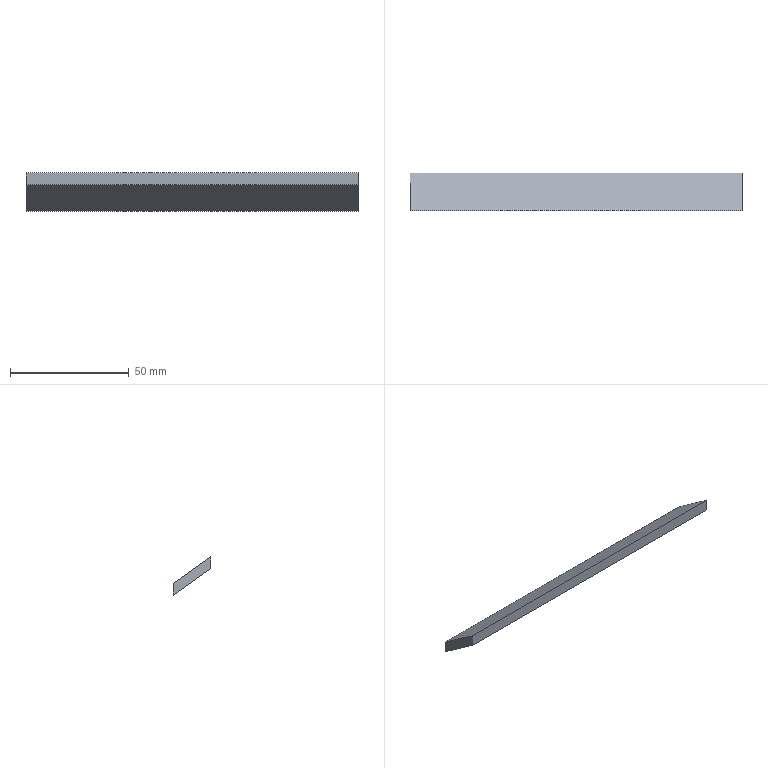Part | STEP file | 06-35 Front-rear dovetail press strip | 1 solid | 6 faces | box 140 x 16 x 16.203 mm | volume 11200 mm3 | plane 6
STEP:
#1=CARTESIAN_POINT('',(0.,0.,0.));
#2=DIRECTION('',(0.,0.,1.));
#3=DIRECTION('',(1.,0.,0.));
#4=AXIS2_PLACEMENT_3D('',#1,#2,#3);
#5=CARTESIAN_POINT('',(140.,0.,-0.000000002));
#6=VERTEX_POINT('',#5);
#7=CARTESIAN_POINT('',(0.,0.,-0.000000001));
#8=VERTEX_POINT('',#7);
#9=CARTESIAN_POINT('',(70.,0.,0.));
#10=DIRECTION('',(-1.,0.,0.));
#11=VECTOR('',#10,1.);
#12=LINE('',#9,#11);
#13=CARTESIAN_POINT('',(0.,0.,0.));
#14=DIRECTION('',(0.,-0.5736,-0.8192));
#15=DIRECTION('',(0.,0.8192,-0.5736));
#16=AXIS2_PLACEMENT_3D('',#13,#14,#15);
#17=PLANE('',#16);
#18=CARTESIAN_POINT('',(0.,70.));
#19=DIRECTION('',(0.,-1.));
#20=VECTOR('',#19,1.);
#21=LINE('',#18,#20);
#22=(GEOMETRIC_REPRESENTATION_CONTEXT(2)PARAMETRIC_REPRESENTATION_CONTEXT()REPRESENTATION_CONTEXT('',''));
#23=DEFINITIONAL_REPRESENTATION('',(#21),#22);
#24=PCURVE('',#17,#23);
#25=CARTESIAN_POINT('',(0.,0.,-5.));
#26=DIRECTION('',(0.,1.,0.));
#27=DIRECTION('',(0.,0.,1.));
#28=AXIS2_PLACEMENT_3D('',#25,#26,#27);
#29=PLANE('',#28);
#30=CARTESIAN_POINT('',(5.,70.));
#31=DIRECTION('',(0.,-1.));
#32=VECTOR('',#31,1.);
#33=LINE('',#30,#32);
#34=(GEOMETRIC_REPRESENTATION_CONTEXT(2)PARAMETRIC_REPRESENTATION_CONTEXT()REPRESENTATION_CONTEXT('',''));
#35=DEFINITIONAL_REPRESENTATION('',(#33),#34);
#36=PCURVE('',#29,#35);
#37=SURFACE_CURVE('',#12,(#24,#36),.PCURVE_S1.);
#38=EDGE_CURVE('',#6,#8,#37,.T.);
#39=ORIENTED_EDGE('',*,*,#38,.F.);
#40=CARTESIAN_POINT('',(140.,16.,-11.203));
#41=VERTEX_POINT('',#40);
#42=CARTESIAN_POINT('',(140.,8.,-5.602));
#43=DIRECTION('',(0.,-0.8192,0.5736));
#44=VECTOR('',#43,1.);
#45=LINE('',#42,#44);
#46=CARTESIAN_POINT('',(9.766,140.));
#47=DIRECTION('',(-1.,0.));
#48=VECTOR('',#47,1.);
#49=LINE('',#46,#48);
#50=(GEOMETRIC_REPRESENTATION_CONTEXT(2)PARAMETRIC_REPRESENTATION_CONTEXT()REPRESENTATION_CONTEXT('',''));
#51=DEFINITIONAL_REPRESENTATION('',(#49),#50);
#52=PCURVE('',#17,#51);
#53=CARTESIAN_POINT('',(140.,0.,0.09722));
#54=DIRECTION('',(1.,0.,0.));
#55=DIRECTION('',(0.,0.,-1.));
#56=AXIS2_PLACEMENT_3D('',#53,#54,#55);
#57=PLANE('',#56);
#58=CARTESIAN_POINT('',(5.699,8.));
#59=DIRECTION('',(-0.5736,-0.8192));
#60=VECTOR('',#59,1.);
#61=LINE('',#58,#60);
#62=(GEOMETRIC_REPRESENTATION_CONTEXT(2)PARAMETRIC_REPRESENTATION_CONTEXT()REPRESENTATION_CONTEXT('',''));
#63=DEFINITIONAL_REPRESENTATION('',(#61),#62);
#64=PCURVE('',#57,#63);
#65=SURFACE_CURVE('',#45,(#52,#64),.PCURVE_S1.);
#66=EDGE_CURVE('',#41,#6,#65,.T.);
#67=ORIENTED_EDGE('',*,*,#66,.F.);
#68=CARTESIAN_POINT('',(0.,16.,-11.203));
#69=VERTEX_POINT('',#68);
#70=CARTESIAN_POINT('',(70.,16.,-11.203));
#71=DIRECTION('',(1.,0.,0.));
#72=VECTOR('',#71,1.);
#73=LINE('',#70,#72);
#74=CARTESIAN_POINT('',(19.532,70.));
#75=DIRECTION('',(0.,1.));
#76=VECTOR('',#75,1.);
#77=LINE('',#74,#76);
#78=(GEOMETRIC_REPRESENTATION_CONTEXT(2)PARAMETRIC_REPRESENTATION_CONTEXT()REPRESENTATION_CONTEXT('',''));
#79=DEFINITIONAL_REPRESENTATION('',(#77),#78);
#80=PCURVE('',#17,#79);
#81=CARTESIAN_POINT('',(0.,16.,-11.203));
#82=DIRECTION('',(0.,-1.,0.));
#83=DIRECTION('',(0.,0.,-1.));
#84=AXIS2_PLACEMENT_3D('',#81,#82,#83);
#85=PLANE('',#84);
#86=CARTESIAN_POINT('',(0.,70.));
#87=DIRECTION('',(0.,1.));
#88=VECTOR('',#87,1.);
#89=LINE('',#86,#88);
#90=(GEOMETRIC_REPRESENTATION_CONTEXT(2)PARAMETRIC_REPRESENTATION_CONTEXT()REPRESENTATION_CONTEXT('',''));
#91=DEFINITIONAL_REPRESENTATION('',(#89),#90);
#92=PCURVE('',#85,#91);
#93=SURFACE_CURVE('',#73,(#80,#92),.PCURVE_S1.);
#94=EDGE_CURVE('',#69,#41,#93,.T.);
#95=ORIENTED_EDGE('',*,*,#94,.F.);
#96=CARTESIAN_POINT('',(0.,8.,-5.602));
#97=DIRECTION('',(0.,0.8192,-0.5736));
#98=VECTOR('',#97,1.);
#99=LINE('',#96,#98);
#100=CARTESIAN_POINT('',(9.766,0.));
#101=DIRECTION('',(1.,0.));
#102=VECTOR('',#101,1.);
#103=LINE('',#100,#102);
#104=(GEOMETRIC_REPRESENTATION_CONTEXT(2)PARAMETRIC_REPRESENTATION_CONTEXT()REPRESENTATION_CONTEXT('',''));
#105=DEFINITIONAL_REPRESENTATION('',(#103),#104);
#106=PCURVE('',#17,#105);
#107=CARTESIAN_POINT('',(0.,0.,0.09722));
#108=DIRECTION('',(1.,0.,0.));
#109=DIRECTION('',(0.,0.,-1.));
#110=AXIS2_PLACEMENT_3D('',#107,#108,#109);
#111=PLANE('',#110);
#112=CARTESIAN_POINT('',(5.699,8.));
#113=DIRECTION('',(0.5736,0.8192));
#114=VECTOR('',#113,1.);
#115=LINE('',#112,#114);
#116=(GEOMETRIC_REPRESENTATION_CONTEXT(2)PARAMETRIC_REPRESENTATION_CONTEXT()REPRESENTATION_CONTEXT('',''));
#117=DEFINITIONAL_REPRESENTATION('',(#115),#116);
#118=PCURVE('',#111,#117);
#119=SURFACE_CURVE('',#99,(#106,#118),.PCURVE_S1.);
#120=EDGE_CURVE('',#8,#69,#119,.T.);
#121=ORIENTED_EDGE('',*,*,#120,.F.);
#122=EDGE_LOOP('',(#39,#67,#95,#121));
#123=FACE_BOUND('',#122,.T.);
#124=ADVANCED_FACE('',(#123),#17,.F.);
#125=CARTESIAN_POINT('',(0.,16.,-16.203));
#126=VERTEX_POINT('',#125);
#127=CARTESIAN_POINT('',(0.,16.,-8.102));
#128=DIRECTION('',(0.,0.,1.));
#129=VECTOR('',#128,1.);
#130=LINE('',#127,#129);
#131=CARTESIAN_POINT('',(8.199,16.));
#132=DIRECTION('',(-1.,0.));
#133=VECTOR('',#132,1.);
#134=LINE('',#131,#133);
#135=(GEOMETRIC_REPRESENTATION_CONTEXT(2)PARAMETRIC_REPRESENTATION_CONTEXT()REPRESENTATION_CONTEXT('',''));
#136=DEFINITIONAL_REPRESENTATION('',(#134),#135);
#137=PCURVE('',#111,#136);
#138=CARTESIAN_POINT('',(-3.102,0.));
#139=DIRECTION('',(-1.,0.));
#140=VECTOR('',#139,1.);
#141=LINE('',#138,#140);
#142=(GEOMETRIC_REPRESENTATION_CONTEXT(2)PARAMETRIC_REPRESENTATION_CONTEXT()REPRESENTATION_CONTEXT('',''));
#143=DEFINITIONAL_REPRESENTATION('',(#141),#142);
#144=PCURVE('',#85,#143);
#145=SURFACE_CURVE('',#130,(#137,#144),.PCURVE_S1.);
#146=EDGE_CURVE('',#126,#69,#145,.T.);
#147=ORIENTED_EDGE('',*,*,#146,.F.);
#148=CARTESIAN_POINT('',(0.,0.,-5.));
#149=VERTEX_POINT('',#148);
#150=CARTESIAN_POINT('',(0.,16.,-16.203));
#151=DIRECTION('',(0.,0.8192,-0.5736));
#152=VECTOR('',#151,1.);
#153=LINE('',#150,#152);
#154=CARTESIAN_POINT('',(16.301,16.));
#155=DIRECTION('',(0.5736,0.8192));
#156=VECTOR('',#155,1.);
#157=LINE('',#154,#156);
#158=(GEOMETRIC_REPRESENTATION_CONTEXT(2)PARAMETRIC_REPRESENTATION_CONTEXT()REPRESENTATION_CONTEXT('',''));
#159=DEFINITIONAL_REPRESENTATION('',(#157),#158);
#160=PCURVE('',#111,#159);
#161=CARTESIAN_POINT('',(0.,16.,-16.203));
#162=DIRECTION('',(0.,0.5736,0.8192));
#163=DIRECTION('',(0.,-0.8192,0.5736));
#164=AXIS2_PLACEMENT_3D('',#161,#162,#163);
#165=PLANE('',#164);
#166=CARTESIAN_POINT('',(0.,0.));
#167=DIRECTION('',(-1.,0.));
#168=VECTOR('',#167,1.);
#169=LINE('',#166,#168);
#170=(GEOMETRIC_REPRESENTATION_CONTEXT(2)PARAMETRIC_REPRESENTATION_CONTEXT()REPRESENTATION_CONTEXT('',''));
#171=DEFINITIONAL_REPRESENTATION('',(#169),#170);
#172=PCURVE('',#165,#171);
#173=SURFACE_CURVE('',#153,(#160,#172),.PCURVE_S1.);
#174=EDGE_CURVE('',#149,#126,#173,.T.);
#175=ORIENTED_EDGE('',*,*,#174,.F.);
#176=CARTESIAN_POINT('',(0.,0.,-8.102));
#177=DIRECTION('',(0.,0.,-1.));
#178=VECTOR('',#177,1.);
#179=LINE('',#176,#178);
#180=CARTESIAN_POINT('',(8.199,0.));
#181=DIRECTION('',(1.,0.));
#182=VECTOR('',#181,1.);
#183=LINE('',#180,#182);
#184=(GEOMETRIC_REPRESENTATION_CONTEXT(2)PARAMETRIC_REPRESENTATION_CONTEXT()REPRESENTATION_CONTEXT('',''));
#185=DEFINITIONAL_REPRESENTATION('',(#183),#184);
#186=PCURVE('',#111,#185);
#187=CARTESIAN_POINT('',(-3.102,0.));
#188=DIRECTION('',(-1.,0.));
#189=VECTOR('',#188,1.);
#190=LINE('',#187,#189);
#191=(GEOMETRIC_REPRESENTATION_CONTEXT(2)PARAMETRIC_REPRESENTATION_CONTEXT()REPRESENTATION_CONTEXT('',''));
#192=DEFINITIONAL_REPRESENTATION('',(#190),#191);
#193=PCURVE('',#29,#192);
#194=SURFACE_CURVE('',#179,(#186,#193),.PCURVE_S1.);
#195=EDGE_CURVE('',#8,#149,#194,.T.);
#196=ORIENTED_EDGE('',*,*,#195,.F.);
#197=ORIENTED_EDGE('',*,*,#120,.T.);
#198=EDGE_LOOP('',(#147,#175,#196,#197));
#199=FACE_BOUND('',#198,.T.);
#200=ADVANCED_FACE('',(#199),#111,.F.);
#201=CARTESIAN_POINT('',(140.,0.,-5.));
#202=VERTEX_POINT('',#201);
#203=CARTESIAN_POINT('',(70.,0.,-5.));
#204=DIRECTION('',(-1.,0.,0.));
#205=VECTOR('',#204,1.);
#206=LINE('',#203,#205);
#207=CARTESIAN_POINT('',(0.,70.));
#208=DIRECTION('',(0.,-1.));
#209=VECTOR('',#208,1.);
#210=LINE('',#207,#209);
#211=(GEOMETRIC_REPRESENTATION_CONTEXT(2)PARAMETRIC_REPRESENTATION_CONTEXT()REPRESENTATION_CONTEXT('',''));
#212=DEFINITIONAL_REPRESENTATION('',(#210),#211);
#213=PCURVE('',#29,#212);
#214=CARTESIAN_POINT('',(19.532,70.));
#215=DIRECTION('',(0.,-1.));
#216=VECTOR('',#215,1.);
#217=LINE('',#214,#216);
#218=(GEOMETRIC_REPRESENTATION_CONTEXT(2)PARAMETRIC_REPRESENTATION_CONTEXT()REPRESENTATION_CONTEXT('',''));
#219=DEFINITIONAL_REPRESENTATION('',(#217),#218);
#220=PCURVE('',#165,#219);
#221=SURFACE_CURVE('',#206,(#213,#220),.PCURVE_S1.);
#222=EDGE_CURVE('',#202,#149,#221,.T.);
#223=ORIENTED_EDGE('',*,*,#222,.F.);
#224=CARTESIAN_POINT('',(140.,0.,-2.5));
#225=DIRECTION('',(0.,0.,-1.));
#226=VECTOR('',#225,1.);
#227=LINE('',#224,#226);
#228=CARTESIAN_POINT('',(2.5,140.));
#229=DIRECTION('',(-1.,0.));
#230=VECTOR('',#229,1.);
#231=LINE('',#228,#230);
#232=(GEOMETRIC_REPRESENTATION_CONTEXT(2)PARAMETRIC_REPRESENTATION_CONTEXT()REPRESENTATION_CONTEXT('',''));
#233=DEFINITIONAL_REPRESENTATION('',(#231),#232);
#234=PCURVE('',#29,#233);
#235=CARTESIAN_POINT('',(2.597,0.));
#236=DIRECTION('',(1.,0.));
#237=VECTOR('',#236,1.);
#238=LINE('',#235,#237);
#239=(GEOMETRIC_REPRESENTATION_CONTEXT(2)PARAMETRIC_REPRESENTATION_CONTEXT()REPRESENTATION_CONTEXT('',''));
#240=DEFINITIONAL_REPRESENTATION('',(#238),#239);
#241=PCURVE('',#57,#240);
#242=SURFACE_CURVE('',#227,(#234,#241),.PCURVE_S1.);
#243=EDGE_CURVE('',#6,#202,#242,.T.);
#244=ORIENTED_EDGE('',*,*,#243,.F.);
#245=ORIENTED_EDGE('',*,*,#38,.T.);
#246=ORIENTED_EDGE('',*,*,#195,.T.);
#247=EDGE_LOOP('',(#223,#244,#245,#246));
#248=FACE_BOUND('',#247,.T.);
#249=ADVANCED_FACE('',(#248),#29,.F.);
#250=CARTESIAN_POINT('',(140.,16.,-16.203));
#251=VERTEX_POINT('',#250);
#252=CARTESIAN_POINT('',(140.,0.,-5.));
#253=DIRECTION('',(0.,0.8192,-0.5736));
#254=VECTOR('',#253,1.);
#255=LINE('',#252,#254);
#256=CARTESIAN_POINT('',(5.097,0.));
#257=DIRECTION('',(0.5736,0.8192));
#258=VECTOR('',#257,1.);
#259=LINE('',#256,#258);
#260=(GEOMETRIC_REPRESENTATION_CONTEXT(2)PARAMETRIC_REPRESENTATION_CONTEXT()REPRESENTATION_CONTEXT('',''));
#261=DEFINITIONAL_REPRESENTATION('',(#259),#260);
#262=PCURVE('',#57,#261);
#263=CARTESIAN_POINT('',(19.532,140.));
#264=DIRECTION('',(-1.,0.));
#265=VECTOR('',#264,1.);
#266=LINE('',#263,#265);
#267=(GEOMETRIC_REPRESENTATION_CONTEXT(2)PARAMETRIC_REPRESENTATION_CONTEXT()REPRESENTATION_CONTEXT('',''));
#268=DEFINITIONAL_REPRESENTATION('',(#266),#267);
#269=PCURVE('',#165,#268);
#270=SURFACE_CURVE('',#255,(#262,#269),.PCURVE_S1.);
#271=EDGE_CURVE('',#202,#251,#270,.T.);
#272=ORIENTED_EDGE('',*,*,#271,.T.);
#273=CARTESIAN_POINT('',(140.,16.,-8.102));
#274=DIRECTION('',(0.,0.,1.));
#275=VECTOR('',#274,1.);
#276=LINE('',#273,#275);
#277=CARTESIAN_POINT('',(8.199,16.));
#278=DIRECTION('',(-1.,0.));
#279=VECTOR('',#278,1.);
#280=LINE('',#277,#279);
#281=(GEOMETRIC_REPRESENTATION_CONTEXT(2)PARAMETRIC_REPRESENTATION_CONTEXT()REPRESENTATION_CONTEXT('',''));
#282=DEFINITIONAL_REPRESENTATION('',(#280),#281);
#283=PCURVE('',#57,#282);
#284=CARTESIAN_POINT('',(-3.102,140.));
#285=DIRECTION('',(-1.,0.));
#286=VECTOR('',#285,1.);
#287=LINE('',#284,#286);
#288=(GEOMETRIC_REPRESENTATION_CONTEXT(2)PARAMETRIC_REPRESENTATION_CONTEXT()REPRESENTATION_CONTEXT('',''));
#289=DEFINITIONAL_REPRESENTATION('',(#287),#288);
#290=PCURVE('',#85,#289);
#291=SURFACE_CURVE('',#276,(#283,#290),.PCURVE_S1.);
#292=EDGE_CURVE('',#251,#41,#291,.T.);
#293=ORIENTED_EDGE('',*,*,#292,.T.);
#294=ORIENTED_EDGE('',*,*,#66,.T.);
#295=ORIENTED_EDGE('',*,*,#243,.T.);
#296=EDGE_LOOP('',(#272,#293,#294,#295));
#297=FACE_BOUND('',#296,.T.);
#298=ADVANCED_FACE('',(#297),#57,.T.);
#299=ORIENTED_EDGE('',*,*,#94,.T.);
#300=ORIENTED_EDGE('',*,*,#292,.F.);
#301=CARTESIAN_POINT('',(70.,16.,-16.203));
#302=DIRECTION('',(1.,0.,0.));
#303=VECTOR('',#302,1.);
#304=LINE('',#301,#303);
#305=CARTESIAN_POINT('',(5.,70.));
#306=DIRECTION('',(0.,1.));
#307=VECTOR('',#306,1.);
#308=LINE('',#305,#307);
#309=(GEOMETRIC_REPRESENTATION_CONTEXT(2)PARAMETRIC_REPRESENTATION_CONTEXT()REPRESENTATION_CONTEXT('',''));
#310=DEFINITIONAL_REPRESENTATION('',(#308),#309);
#311=PCURVE('',#85,#310);
#312=CARTESIAN_POINT('',(0.,70.));
#313=DIRECTION('',(0.,1.));
#314=VECTOR('',#313,1.);
#315=LINE('',#312,#314);
#316=(GEOMETRIC_REPRESENTATION_CONTEXT(2)PARAMETRIC_REPRESENTATION_CONTEXT()REPRESENTATION_CONTEXT('',''));
#317=DEFINITIONAL_REPRESENTATION('',(#315),#316);
#318=PCURVE('',#165,#317);
#319=SURFACE_CURVE('',#304,(#311,#318),.PCURVE_S1.);
#320=EDGE_CURVE('',#126,#251,#319,.T.);
#321=ORIENTED_EDGE('',*,*,#320,.F.);
#322=ORIENTED_EDGE('',*,*,#146,.T.);
#323=EDGE_LOOP('',(#299,#300,#321,#322));
#324=FACE_BOUND('',#323,.T.);
#325=ADVANCED_FACE('',(#324),#85,.F.);
#326=ORIENTED_EDGE('',*,*,#320,.T.);
#327=ORIENTED_EDGE('',*,*,#271,.F.);
#328=ORIENTED_EDGE('',*,*,#222,.T.);
#329=ORIENTED_EDGE('',*,*,#174,.T.);
#330=EDGE_LOOP('',(#326,#327,#328,#329));
#331=FACE_BOUND('',#330,.T.);
#332=ADVANCED_FACE('',(#331),#165,.F.);
#333=CLOSED_SHELL('',(#124,#200,#249,#298,#325,#332));
#334=MANIFOLD_SOLID_BREP('',#333);
#335=(LENGTH_UNIT()NAMED_UNIT(*)SI_UNIT(.MILLI.,.METRE.));
#336=UNCERTAINTY_MEASURE_WITH_UNIT(LENGTH_MEASURE(0.0000001),#335,'','');
#337=(NAMED_UNIT(*)PLANE_ANGLE_UNIT()SI_UNIT($,.RADIAN.));
#338=(NAMED_UNIT(*)SI_UNIT($,.STERADIAN.)SOLID_ANGLE_UNIT());
#339=(GEOMETRIC_REPRESENTATION_CONTEXT(3)GLOBAL_UNCERTAINTY_ASSIGNED_CONTEXT((#336))GLOBAL_UNIT_ASSIGNED_CONTEXT((#335,#337,#338))REPRESENTATION_CONTEXT('',''));
#340=ADVANCED_BREP_SHAPE_REPRESENTATION('',(#4,#334),#339);